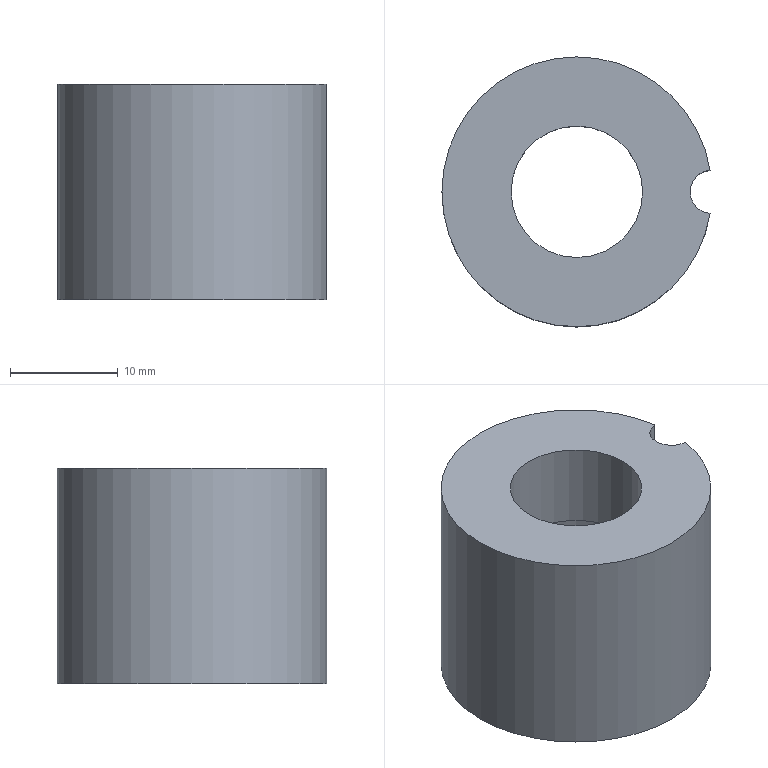Part | NX | features solid 2 | 1 solid | 7 faces | box 24.84 x 25 x 20 mm | volume 6165 mm3 | cylinder 4 | plane 3 | commonest cylinder face diameters 4 x1 12.19 x1 16.6 x1 25 x1
STEP:
#1=CARTESIAN_POINT('',(-306.734,-431.497,97.308));
#2=VERTEX_POINT('',#1);
#3=CARTESIAN_POINT('',(-306.734,-427.51,97.308));
#4=VERTEX_POINT('',#3);
#5=CARTESIAN_POINT('',(-306.574,-429.504,97.308));
#6=DIRECTION('',(0.,0.,-1.));
#7=DIRECTION('',(-1.,0.,0.));
#8=AXIS2_PLACEMENT_3D('',#5,#6,#7);
#9=CIRCLE('',#8,2.);
#10=EDGE_CURVE('',#2,#4,#9,.T.);
#11=ORIENTED_EDGE('',*,*,#10,.T.);
#12=CARTESIAN_POINT('',(-319.074,-429.504,97.308));
#13=DIRECTION('',(0.,0.,-1.));
#14=DIRECTION('',(-1.,0.,0.));
#15=AXIS2_PLACEMENT_3D('',#12,#13,#14);
#16=CIRCLE('',#15,12.5);
#17=EDGE_CURVE('',#2,#4,#16,.T.);
#18=ORIENTED_EDGE('',*,*,#17,.F.);
#19=EDGE_LOOP('',(#11,#18));
#20=FACE_BOUND('',#19,.T.);
#21=CARTESIAN_POINT('',(-325.169,-429.504,97.308));
#22=VERTEX_POINT('',#21);
#23=CARTESIAN_POINT('',(-319.074,-429.504,97.308));
#24=DIRECTION('',(0.,0.,-1.));
#25=DIRECTION('',(-1.,0.,0.));
#26=AXIS2_PLACEMENT_3D('',#23,#24,#25);
#27=CIRCLE('',#26,6.095);
#28=EDGE_CURVE('',#22,#22,#27,.T.);
#29=ORIENTED_EDGE('',*,*,#28,.T.);
#30=EDGE_LOOP('',(#29));
#31=FACE_BOUND('',#30,.T.);
#32=CARTESIAN_POINT('',(-319.074,-429.504,97.308));
#33=DIRECTION('',(0.,0.,1.));
#34=DIRECTION('',(1.,0.,0.));
#35=AXIS2_PLACEMENT_3D('',#32,#33,#34);
#36=PLANE('',#35);
#37=ADVANCED_FACE('',(#20,#31),#36,.T.);
#38=CARTESIAN_POINT('',(-306.734,-427.51,77.308));
#39=VERTEX_POINT('',#38);
#40=CARTESIAN_POINT('',(-306.734,-431.497,77.308));
#41=VERTEX_POINT('',#40);
#42=CARTESIAN_POINT('',(-306.574,-429.504,77.308));
#43=DIRECTION('',(0.,0.,1.));
#44=DIRECTION('',(1.,0.,0.));
#45=AXIS2_PLACEMENT_3D('',#42,#43,#44);
#46=CIRCLE('',#45,2.);
#47=EDGE_CURVE('',#39,#41,#46,.T.);
#48=ORIENTED_EDGE('',*,*,#47,.T.);
#49=CARTESIAN_POINT('',(-319.074,-429.504,77.308));
#50=DIRECTION('',(0.,0.,1.));
#51=DIRECTION('',(1.,0.,0.));
#52=AXIS2_PLACEMENT_3D('',#49,#50,#51);
#53=CIRCLE('',#52,12.5);
#54=EDGE_CURVE('',#39,#41,#53,.T.);
#55=ORIENTED_EDGE('',*,*,#54,.F.);
#56=EDGE_LOOP('',(#48,#55));
#57=FACE_BOUND('',#56,.T.);
#58=CARTESIAN_POINT('',(-310.774,-429.504,77.308));
#59=VERTEX_POINT('',#58);
#60=CARTESIAN_POINT('',(-319.074,-429.504,77.308));
#61=DIRECTION('',(0.,0.,1.));
#62=DIRECTION('',(1.,0.,0.));
#63=AXIS2_PLACEMENT_3D('',#60,#61,#62);
#64=CIRCLE('',#63,8.3);
#65=EDGE_CURVE('',#59,#59,#64,.T.);
#66=ORIENTED_EDGE('',*,*,#65,.T.);
#67=EDGE_LOOP('',(#66));
#68=FACE_BOUND('',#67,.T.);
#69=CARTESIAN_POINT('',(-319.074,-429.504,77.308));
#70=DIRECTION('',(0.,0.,-1.));
#71=DIRECTION('',(-1.,0.,0.));
#72=AXIS2_PLACEMENT_3D('',#69,#70,#71);
#73=PLANE('',#72);
#74=ADVANCED_FACE('',(#57,#68),#73,.T.);
#75=CARTESIAN_POINT('',(-306.734,-427.51,87.308));
#76=DIRECTION('',(0.,0.,1.));
#77=VECTOR('',#76,1000.);
#78=LINE('',#75,#77);
#79=EDGE_CURVE('',#39,#4,#78,.T.);
#80=ORIENTED_EDGE('',*,*,#79,.F.);
#81=ORIENTED_EDGE('',*,*,#54,.T.);
#82=CARTESIAN_POINT('',(-306.734,-431.497,87.308));
#83=DIRECTION('',(0.,0.,1.));
#84=VECTOR('',#83,1000.);
#85=LINE('',#82,#84);
#86=EDGE_CURVE('',#2,#41,#85,.F.);
#87=ORIENTED_EDGE('',*,*,#86,.F.);
#88=ORIENTED_EDGE('',*,*,#17,.T.);
#89=EDGE_LOOP('',(#80,#81,#87,#88));
#90=FACE_BOUND('',#89,.T.);
#91=CARTESIAN_POINT('',(-319.074,-429.504,77.308));
#92=DIRECTION('',(0.,0.,1.));
#93=DIRECTION('',(1.,0.,0.));
#94=AXIS2_PLACEMENT_3D('',#91,#92,#93);
#95=CYLINDRICAL_SURFACE('',#94,12.5);
#96=ADVANCED_FACE('',(#90),#95,.T.);
#97=CARTESIAN_POINT('',(-312.979,-429.504,89.308));
#98=VERTEX_POINT('',#97);
#99=CARTESIAN_POINT('',(-319.074,-429.504,89.308));
#100=DIRECTION('',(0.,0.,1.));
#101=DIRECTION('',(1.,0.,0.));
#102=AXIS2_PLACEMENT_3D('',#99,#100,#101);
#103=CIRCLE('',#102,6.095);
#104=EDGE_CURVE('',#98,#98,#103,.T.);
#105=ORIENTED_EDGE('',*,*,#104,.T.);
#106=EDGE_LOOP('',(#105));
#107=FACE_BOUND('',#106,.T.);
#108=CARTESIAN_POINT('',(-327.374,-429.504,89.308));
#109=VERTEX_POINT('',#108);
#110=CARTESIAN_POINT('',(-319.074,-429.504,89.308));
#111=DIRECTION('',(0.,0.,-1.));
#112=DIRECTION('',(-1.,0.,0.));
#113=AXIS2_PLACEMENT_3D('',#110,#111,#112);
#114=CIRCLE('',#113,8.3);
#115=EDGE_CURVE('',#109,#109,#114,.T.);
#116=ORIENTED_EDGE('',*,*,#115,.T.);
#117=EDGE_LOOP('',(#116));
#118=FACE_BOUND('',#117,.T.);
#119=CARTESIAN_POINT('',(-319.074,-429.504,89.308));
#120=DIRECTION('',(0.,0.,1.));
#121=DIRECTION('',(1.,0.,0.));
#122=AXIS2_PLACEMENT_3D('',#119,#120,#121);
#123=PLANE('',#122);
#124=ADVANCED_FACE('',(#107,#118),#123,.F.);
#125=ORIENTED_EDGE('',*,*,#115,.F.);
#126=EDGE_LOOP('',(#125));
#127=FACE_BOUND('',#126,.T.);
#128=ORIENTED_EDGE('',*,*,#65,.F.);
#129=EDGE_LOOP('',(#128));
#130=FACE_BOUND('',#129,.T.);
#131=CARTESIAN_POINT('',(-319.074,-429.504,77.308));
#132=DIRECTION('',(0.,0.,1.));
#133=DIRECTION('',(1.,0.,0.));
#134=AXIS2_PLACEMENT_3D('',#131,#132,#133);
#135=CYLINDRICAL_SURFACE('',#134,8.3);
#136=ADVANCED_FACE('',(#127,#130),#135,.F.);
#137=ORIENTED_EDGE('',*,*,#28,.F.);
#138=EDGE_LOOP('',(#137));
#139=FACE_BOUND('',#138,.T.);
#140=ORIENTED_EDGE('',*,*,#104,.F.);
#141=EDGE_LOOP('',(#140));
#142=FACE_BOUND('',#141,.T.);
#143=CARTESIAN_POINT('',(-319.074,-429.504,89.308));
#144=DIRECTION('',(0.,0.,1.));
#145=DIRECTION('',(1.,0.,0.));
#146=AXIS2_PLACEMENT_3D('',#143,#144,#145);
#147=CYLINDRICAL_SURFACE('',#146,6.095);
#148=ADVANCED_FACE('',(#139,#142),#147,.F.);
#149=ORIENTED_EDGE('',*,*,#79,.T.);
#150=ORIENTED_EDGE('',*,*,#10,.F.);
#151=ORIENTED_EDGE('',*,*,#86,.T.);
#152=ORIENTED_EDGE('',*,*,#47,.F.);
#153=EDGE_LOOP('',(#149,#150,#151,#152));
#154=FACE_BOUND('',#153,.T.);
#155=CARTESIAN_POINT('',(-306.574,-429.504,77.308));
#156=DIRECTION('',(0.,0.,1.));
#157=DIRECTION('',(1.,0.,0.));
#158=AXIS2_PLACEMENT_3D('',#155,#156,#157);
#159=CYLINDRICAL_SURFACE('',#158,2.);
#160=ADVANCED_FACE('',(#154),#159,.F.);
#161=CLOSED_SHELL('',(#37,#74,#96,#124,#136,#148,#160));
#162=MANIFOLD_SOLID_BREP('',#161);
#163=(LENGTH_UNIT()NAMED_UNIT(*)SI_UNIT(.MILLI.,.METRE.));
#164=UNCERTAINTY_MEASURE_WITH_UNIT(LENGTH_MEASURE(0.00001),#163,'','');
#165=(NAMED_UNIT(*)PLANE_ANGLE_UNIT()SI_UNIT($,.RADIAN.));
#166=(NAMED_UNIT(*)SI_UNIT($,.STERADIAN.)SOLID_ANGLE_UNIT());
#167=(GEOMETRIC_REPRESENTATION_CONTEXT(3)GLOBAL_UNCERTAINTY_ASSIGNED_CONTEXT((#164))GLOBAL_UNIT_ASSIGNED_CONTEXT((#163,#165,#166))REPRESENTATION_CONTEXT('',''));
#168=ADVANCED_BREP_SHAPE_REPRESENTATION('',(#162),#167);